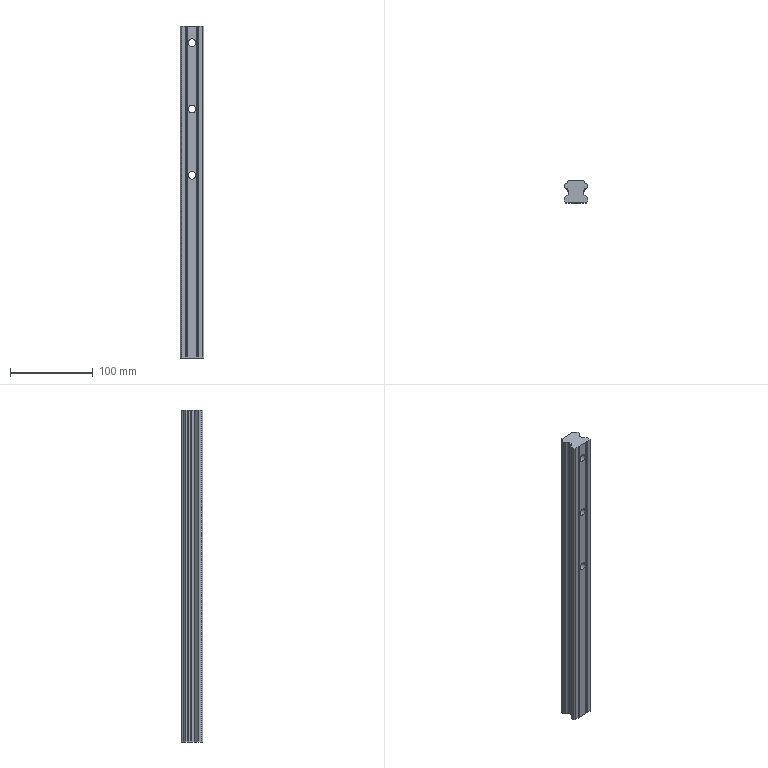Part | SolidWorks | features BaseBody 1, ICE 1 | 1 solid | 67 faces | box 28 x 26 x 400 mm | volume 237087 mm3 | cylinder 34 | plane 33 | commonest cylinder face diameters 1.2 x12 1.6 x6 9 x6 14 x6 5.66 x4